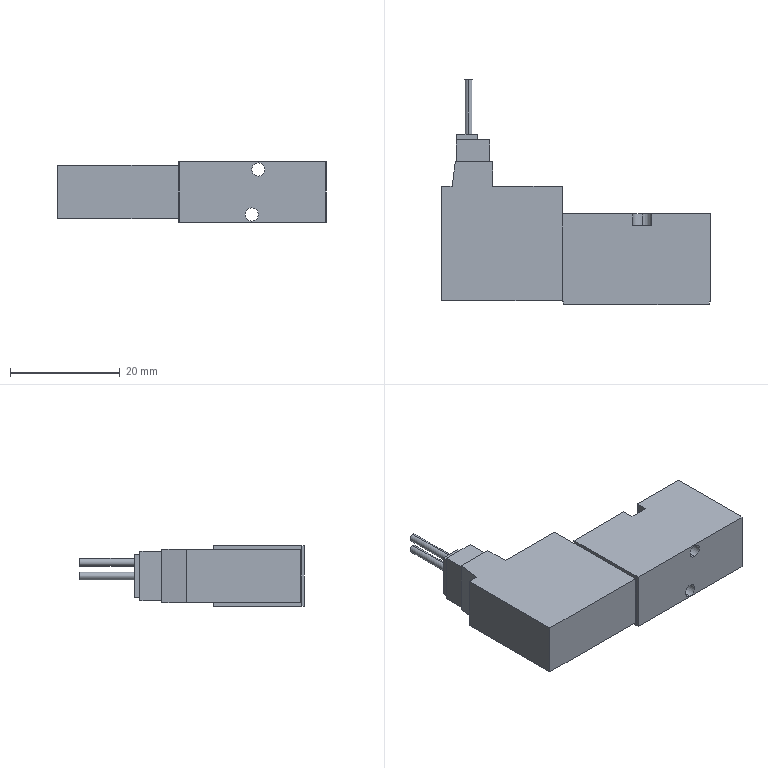Part | SolidWorks | features BaseBody 1, ICE 1 | 1 solid | 49 faces | box 49 x 41 x 11 mm | volume 9805 mm3 | plane 34 | cylinder 11 | spline 4 | commonest cylinder face diameters 1.4 x4 2.4 x4 3.5 x3
STEP:
#1=CARTESIAN_POINT('',(-0.6,14.4,-5.3));
#2=VERTEX_POINT('',#1);
#3=CARTESIAN_POINT('',(-0.6,14.4,-2.9));
#4=VERTEX_POINT('',#3);
#5=CARTESIAN_POINT('',(-0.6,14.4,-4.1));
#6=DIRECTION('',(0.,1.,0.));
#7=DIRECTION('',(0.,0.,-1.));
#8=AXIS2_PLACEMENT_3D('',#5,#6,#7);
#9=CIRCLE('',#8,1.2);
#10=EDGE_CURVE('',#2,#4,#9,.T.);
#11=ORIENTED_EDGE('',*,*,#10,.T.);
#12=CARTESIAN_POINT('',(-0.6,0.,-2.9));
#13=VERTEX_POINT('',#12);
#14=CARTESIAN_POINT('',(-0.6,14.4,-2.9));
#15=DIRECTION('',(0.,-1.,0.));
#16=VECTOR('',#15,1000.);
#17=LINE('',#14,#16);
#18=EDGE_CURVE('',#4,#13,#17,.T.);
#19=ORIENTED_EDGE('',*,*,#18,.T.);
#20=CARTESIAN_POINT('',(-0.6,0.,-5.3));
#21=VERTEX_POINT('',#20);
#22=CARTESIAN_POINT('',(-0.6,0.,-4.1));
#23=DIRECTION('',(0.,1.,0.));
#24=DIRECTION('',(0.,0.,1.));
#25=AXIS2_PLACEMENT_3D('',#22,#23,#24);
#26=CIRCLE('',#25,1.2);
#27=EDGE_CURVE('',#21,#13,#26,.T.);
#28=ORIENTED_EDGE('',*,*,#27,.F.);
#29=CARTESIAN_POINT('',(-0.6,14.4,-5.3));
#30=DIRECTION('',(0.,-1.,0.));
#31=VECTOR('',#30,1000.);
#32=LINE('',#29,#31);
#33=EDGE_CURVE('',#2,#21,#32,.T.);
#34=ORIENTED_EDGE('',*,*,#33,.F.);
#35=EDGE_LOOP('',(#11,#19,#28,#34));
#36=FACE_OUTER_BOUND('',#35,.T.);
#37=CARTESIAN_POINT('',(-0.6,14.4,-4.1));
#38=DIRECTION('',(0.,-1.,0.));
#39=DIRECTION('',(0.,0.,-1.));
#40=AXIS2_PLACEMENT_3D('',#37,#38,#39);
#41=CYLINDRICAL_SURFACE('',#40,1.2);
#42=ADVANCED_FACE('',(#36),#41,.F.);
#43=CARTESIAN_POINT('',(0.6,16.5,2.35));
#44=VERTEX_POINT('',#43);
#45=CARTESIAN_POINT('',(2.35,16.5,4.1));
#46=VERTEX_POINT('',#45);
#47=CARTESIAN_POINT('',(0.6,16.5,4.1));
#48=DIRECTION('',(0.,-1.,0.));
#49=DIRECTION('',(0.,0.,-1.));
#50=AXIS2_PLACEMENT_3D('',#47,#48,#49);
#51=CIRCLE('',#50,1.75);
#52=EDGE_CURVE('',#44,#46,#51,.T.);
#53=ORIENTED_EDGE('',*,*,#52,.F.);
#54=CARTESIAN_POINT('',(0.6,14.4,2.35));
#55=VERTEX_POINT('',#54);
#56=CARTESIAN_POINT('',(0.6,16.5,2.35));
#57=DIRECTION('',(0.,-1.,0.));
#58=VECTOR('',#57,1000.);
#59=LINE('',#56,#58);
#60=EDGE_CURVE('',#44,#55,#59,.T.);
#61=ORIENTED_EDGE('',*,*,#60,.T.);
#62=CARTESIAN_POINT('',(2.35,14.4,4.1));
#63=VERTEX_POINT('',#62);
#64=CARTESIAN_POINT('',(0.6,14.4,4.1));
#65=DIRECTION('',(0.,-1.,0.));
#66=DIRECTION('',(0.,0.,-1.));
#67=AXIS2_PLACEMENT_3D('',#64,#65,#66);
#68=CIRCLE('',#67,1.75);
#69=EDGE_CURVE('',#55,#63,#68,.T.);
#70=ORIENTED_EDGE('',*,*,#69,.T.);
#71=CARTESIAN_POINT('',(2.35,15.45,4.1));
#72=DIRECTION('',(0.,1.,0.));
#73=VECTOR('',#72,1000.);
#74=LINE('',#71,#73);
#75=EDGE_CURVE('',#63,#46,#74,.T.);
#76=ORIENTED_EDGE('',*,*,#75,.T.);
#77=EDGE_LOOP('',(#53,#61,#70,#76));
#78=FACE_OUTER_BOUND('',#77,.T.);
#79=CARTESIAN_POINT('',(0.6,16.5,4.1));
#80=DIRECTION('',(0.,-1.,0.));
#81=DIRECTION('',(0.,0.,-1.));
#82=AXIS2_PLACEMENT_3D('',#79,#80,#81);
#83=CYLINDRICAL_SURFACE('',#82,1.75);
#84=ADVANCED_FACE('',(#78),#83,.F.);
#85=CARTESIAN_POINT('',(0.6,14.4,5.3));
#86=VERTEX_POINT('',#85);
#87=CARTESIAN_POINT('',(0.6,14.4,2.9));
#88=VERTEX_POINT('',#87);
#89=CARTESIAN_POINT('',(0.6,14.4,4.1));
#90=DIRECTION('',(0.,-1.,0.));
#91=DIRECTION('',(0.,0.,-1.));
#92=AXIS2_PLACEMENT_3D('',#89,#90,#91);
#93=CIRCLE('',#92,1.2);
#94=EDGE_CURVE('',#86,#88,#93,.T.);
#95=ORIENTED_EDGE('',*,*,#94,.F.);
#96=CARTESIAN_POINT('',(0.6,0.,5.3));
#97=VERTEX_POINT('',#96);
#98=CARTESIAN_POINT('',(0.6,14.4,5.3));
#99=DIRECTION('',(0.,-1.,0.));
#100=VECTOR('',#99,1000.);
#101=LINE('',#98,#100);
#102=EDGE_CURVE('',#86,#97,#101,.T.);
#103=ORIENTED_EDGE('',*,*,#102,.T.);
#104=CARTESIAN_POINT('',(0.6,0.,2.9));
#105=VERTEX_POINT('',#104);
#106=CARTESIAN_POINT('',(0.6,0.,4.1));
#107=DIRECTION('',(0.,1.,0.));
#108=DIRECTION('',(0.,0.,1.));
#109=AXIS2_PLACEMENT_3D('',#106,#107,#108);
#110=CIRCLE('',#109,1.2);
#111=EDGE_CURVE('',#105,#97,#110,.T.);
#112=ORIENTED_EDGE('',*,*,#111,.F.);
#113=CARTESIAN_POINT('',(0.6,14.4,2.9));
#114=DIRECTION('',(0.,-1.,0.));
#115=VECTOR('',#114,1000.);
#116=LINE('',#113,#115);
#117=EDGE_CURVE('',#88,#105,#116,.T.);
#118=ORIENTED_EDGE('',*,*,#117,.F.);
#119=EDGE_LOOP('',(#95,#103,#112,#118));
#120=FACE_OUTER_BOUND('',#119,.T.);
#121=CARTESIAN_POINT('',(0.6,14.4,4.1));
#122=DIRECTION('',(0.,-1.,0.));
#123=DIRECTION('',(0.,0.,-1.));
#124=AXIS2_PLACEMENT_3D('',#121,#122,#123);
#125=CYLINDRICAL_SURFACE('',#124,1.2);
#126=ADVANCED_FACE('',(#120),#125,.F.);
#127=CARTESIAN_POINT('',(-31.07,31.,-0.7));
#128=VERTEX_POINT('',#127);
#129=CARTESIAN_POINT('',(-31.07,31.,0.7));
#130=VERTEX_POINT('',#129);
#131=CARTESIAN_POINT('',(-31.07,31.,0.));
#132=DIRECTION('',(0.,-1.,0.));
#133=DIRECTION('',(0.,0.,1.));
#134=AXIS2_PLACEMENT_3D('',#131,#132,#133);
#135=CIRCLE('',#134,0.7);
#136=EDGE_CURVE('',#128,#130,#135,.T.);
#137=ORIENTED_EDGE('',*,*,#136,.F.);
#138=CARTESIAN_POINT('',(-31.07,41.,-0.7));
#139=VERTEX_POINT('',#138);
#140=CARTESIAN_POINT('',(-31.07,41.,-0.7));
#141=DIRECTION('',(0.,1.,0.));
#142=VECTOR('',#141,1000.);
#143=LINE('',#140,#142);
#144=EDGE_CURVE('',#128,#139,#143,.T.);
#145=ORIENTED_EDGE('',*,*,#144,.T.);
#146=CARTESIAN_POINT('',(-31.07,41.,0.7));
#147=VERTEX_POINT('',#146);
#148=CARTESIAN_POINT('',(-31.07,41.,0.));
#149=DIRECTION('',(0.,-1.,0.));
#150=DIRECTION('',(0.,0.,1.));
#151=AXIS2_PLACEMENT_3D('',#148,#149,#150);
#152=CIRCLE('',#151,0.7);
#153=EDGE_CURVE('',#139,#147,#152,.T.);
#154=ORIENTED_EDGE('',*,*,#153,.T.);
#155=CARTESIAN_POINT('',(-31.07,41.,0.7));
#156=DIRECTION('',(0.,1.,0.));
#157=VECTOR('',#156,1000.);
#158=LINE('',#155,#157);
#159=EDGE_CURVE('',#130,#147,#158,.T.);
#160=ORIENTED_EDGE('',*,*,#159,.F.);
#161=EDGE_LOOP('',(#137,#145,#154,#160));
#162=FACE_OUTER_BOUND('',#161,.T.);
#163=CARTESIAN_POINT('',(-31.07,41.,0.));
#164=DIRECTION('',(0.,1.,0.));
#165=DIRECTION('',(0.,0.,1.));
#166=AXIS2_PLACEMENT_3D('',#163,#164,#165);
#167=CYLINDRICAL_SURFACE('',#166,0.7);
#168=ADVANCED_FACE('',(#162),#167,.T.);
#169=CARTESIAN_POINT('',(-31.07,31.,1.8));
#170=VERTEX_POINT('',#169);
#171=CARTESIAN_POINT('',(-31.07,31.,3.2));
#172=VERTEX_POINT('',#171);
#173=CARTESIAN_POINT('',(-31.07,31.,2.5));
#174=DIRECTION('',(0.,-1.,0.));
#175=DIRECTION('',(0.,0.,1.));
#176=AXIS2_PLACEMENT_3D('',#173,#174,#175);
#177=CIRCLE('',#176,0.7);
#178=EDGE_CURVE('',#170,#172,#177,.T.);
#179=ORIENTED_EDGE('',*,*,#178,.F.);
#180=CARTESIAN_POINT('',(-31.07,41.,1.8));
#181=VERTEX_POINT('',#180);
#182=CARTESIAN_POINT('',(-31.07,41.,1.8));
#183=DIRECTION('',(0.,1.,0.));
#184=VECTOR('',#183,1000.);
#185=LINE('',#182,#184);
#186=EDGE_CURVE('',#170,#181,#185,.T.);
#187=ORIENTED_EDGE('',*,*,#186,.T.);
#188=CARTESIAN_POINT('',(-31.07,41.,3.2));
#189=VERTEX_POINT('',#188);
#190=CARTESIAN_POINT('',(-31.07,41.,2.5));
#191=DIRECTION('',(0.,-1.,0.));
#192=DIRECTION('',(0.,0.,1.));
#193=AXIS2_PLACEMENT_3D('',#190,#191,#192);
#194=CIRCLE('',#193,0.7);
#195=EDGE_CURVE('',#181,#189,#194,.T.);
#196=ORIENTED_EDGE('',*,*,#195,.T.);
#197=CARTESIAN_POINT('',(-31.07,41.,3.2));
#198=DIRECTION('',(0.,1.,0.));
#199=VECTOR('',#198,1000.);
#200=LINE('',#197,#199);
#201=EDGE_CURVE('',#172,#189,#200,.T.);
#202=ORIENTED_EDGE('',*,*,#201,.F.);
#203=EDGE_LOOP('',(#179,#187,#196,#202));
#204=FACE_OUTER_BOUND('',#203,.T.);
#205=CARTESIAN_POINT('',(-31.07,41.,2.5));
#206=DIRECTION('',(0.,1.,0.));
#207=DIRECTION('',(0.,0.,1.));
#208=AXIS2_PLACEMENT_3D('',#205,#206,#207);
#209=CYLINDRICAL_SURFACE('',#208,0.7);
#210=ADVANCED_FACE('',(#204),#209,.T.);
#211=ORIENTED_EDGE('',*,*,#18,.F.);
#212=CARTESIAN_POINT('',(-0.6,14.4,-4.1));
#213=DIRECTION('',(0.,1.,0.));
#214=DIRECTION('',(0.,0.,-1.));
#215=AXIS2_PLACEMENT_3D('',#212,#213,#214);
#216=CIRCLE('',#215,1.2);
#217=EDGE_CURVE('',#4,#2,#216,.T.);
#218=ORIENTED_EDGE('',*,*,#217,.T.);
#219=ORIENTED_EDGE('',*,*,#33,.T.);
#220=CARTESIAN_POINT('',(-0.6,0.,-4.1));
#221=DIRECTION('',(0.,1.,0.));
#222=DIRECTION('',(0.,0.,1.));
#223=AXIS2_PLACEMENT_3D('',#220,#221,#222);
#224=CIRCLE('',#223,1.2);
#225=EDGE_CURVE('',#13,#21,#224,.T.);
#226=ORIENTED_EDGE('',*,*,#225,.F.);
#227=EDGE_LOOP('',(#211,#218,#219,#226));
#228=FACE_OUTER_BOUND('',#227,.T.);
#229=CARTESIAN_POINT('',(-0.6,14.4,-4.1));
#230=DIRECTION('',(0.,-1.,0.));
#231=DIRECTION('',(0.,0.,-1.));
#232=AXIS2_PLACEMENT_3D('',#229,#230,#231);
#233=CYLINDRICAL_SURFACE('',#232,1.2);
#234=ADVANCED_FACE('',(#228),#233,.F.);
#235=ORIENTED_EDGE('',*,*,#10,.F.);
#236=ORIENTED_EDGE('',*,*,#217,.F.);
#237=EDGE_LOOP('',(#235,#236));
#238=FACE_BOUND('',#237,.T.);
#239=CARTESIAN_POINT('',(1.15,14.4,-5.5));
#240=VERTEX_POINT('',#239);
#241=CARTESIAN_POINT('',(-2.35,14.4,-5.5));
#242=VERTEX_POINT('',#241);
#243=CARTESIAN_POINT('',(-2.35,14.4,-5.5));
#244=DIRECTION('',(-1.,0.,0.));
#245=VECTOR('',#244,1000.);
#246=LINE('',#243,#245);
#247=EDGE_CURVE('',#240,#242,#246,.T.);
#248=ORIENTED_EDGE('',*,*,#247,.T.);
#249=CARTESIAN_POINT('',(-2.35,14.4,-4.1));
#250=VERTEX_POINT('',#249);
#251=CARTESIAN_POINT('',(-2.35,14.4,-4.8));
#252=DIRECTION('',(0.,0.,-1.));
#253=VECTOR('',#252,1000.);
#254=LINE('',#251,#253);
#255=EDGE_CURVE('',#250,#242,#254,.T.);
#256=ORIENTED_EDGE('',*,*,#255,.F.);
#257=CARTESIAN_POINT('',(1.15,14.4,-4.1));
#258=VERTEX_POINT('',#257);
#259=CARTESIAN_POINT('',(-0.6,14.4,-4.1));
#260=DIRECTION('',(0.,1.,0.));
#261=DIRECTION('',(0.,0.,-1.));
#262=AXIS2_PLACEMENT_3D('',#259,#260,#261);
#263=CIRCLE('',#262,1.75);
#264=EDGE_CURVE('',#250,#258,#263,.T.);
#265=ORIENTED_EDGE('',*,*,#264,.T.);
#266=CARTESIAN_POINT('',(1.15,14.4,-4.8));
#267=DIRECTION('',(0.,0.,1.));
#268=VECTOR('',#267,1000.);
#269=LINE('',#266,#268);
#270=EDGE_CURVE('',#240,#258,#269,.T.);
#271=ORIENTED_EDGE('',*,*,#270,.F.);
#272=EDGE_LOOP('',(#248,#256,#265,#271));
#273=FACE_OUTER_BOUND('',#272,.T.);
#274=CARTESIAN_POINT('',(-2.35,14.4,-5.5));
#275=CARTESIAN_POINT('',(1.15,14.4,-5.5));
#276=CARTESIAN_POINT('',(-2.35,14.4,-2.35));
#277=CARTESIAN_POINT('',(1.15,14.4,-2.35));
#278=CARTESIAN_POINT('',(-2.35,14.4,-2.322));
#279=CARTESIAN_POINT('',(1.15,14.4,-2.322));
#280=B_SPLINE_SURFACE_WITH_KNOTS('',1,1,((#274,#275),(#276,#277),(#278,#279)),.UNSPECIFIED.,.F.,.F.,.F.,(2,1,2),(2,2),(0.,1.,1.009),(0.,1.),.UNSPECIFIED.);
#281=ADVANCED_FACE('',(#238,#273),#280,.T.);
#282=CARTESIAN_POINT('',(-14.,0.5,-5.5));
#283=VERTEX_POINT('',#282);
#284=CARTESIAN_POINT('',(-14.,16.5,-5.5));
#285=VERTEX_POINT('',#284);
#286=CARTESIAN_POINT('',(-14.,0.,-5.5));
#287=DIRECTION('',(0.,1.,0.));
#288=VECTOR('',#287,1000.);
#289=LINE('',#286,#288);
#290=EDGE_CURVE('',#283,#285,#289,.T.);
#291=ORIENTED_EDGE('',*,*,#290,.T.);
#292=CARTESIAN_POINT('',(-2.35,16.5,-5.5));
#293=VERTEX_POINT('',#292);
#294=CARTESIAN_POINT('',(-0.5,16.5,-5.5));
#295=DIRECTION('',(1.,0.,0.));
#296=VECTOR('',#295,1000.);
#297=LINE('',#294,#296);
#298=EDGE_CURVE('',#285,#293,#297,.T.);
#299=ORIENTED_EDGE('',*,*,#298,.T.);
#300=CARTESIAN_POINT('',(-2.35,0.,-5.5));
#301=DIRECTION('',(0.,-1.,0.));
#302=VECTOR('',#301,1000.);
#303=LINE('',#300,#302);
#304=EDGE_CURVE('',#293,#242,#303,.T.);
#305=ORIENTED_EDGE('',*,*,#304,.T.);
#306=ORIENTED_EDGE('',*,*,#247,.F.);
#307=CARTESIAN_POINT('',(1.15,16.5,-5.5));
#308=VERTEX_POINT('',#307);
#309=CARTESIAN_POINT('',(1.15,0.,-5.5));
#310=DIRECTION('',(0.,1.,0.));
#311=VECTOR('',#310,1000.);
#312=LINE('',#309,#311);
#313=EDGE_CURVE('',#240,#308,#312,.T.);
#314=ORIENTED_EDGE('',*,*,#313,.T.);
#315=CARTESIAN_POINT('',(13.,16.5,-5.5));
#316=VERTEX_POINT('',#315);
#317=CARTESIAN_POINT('',(-0.5,16.5,-5.5));
#318=DIRECTION('',(1.,0.,0.));
#319=VECTOR('',#318,1000.);
#320=LINE('',#317,#319);
#321=EDGE_CURVE('',#308,#316,#320,.T.);
#322=ORIENTED_EDGE('',*,*,#321,.T.);
#323=CARTESIAN_POINT('',(13.,0.5,-5.5));
#324=VERTEX_POINT('',#323);
#325=CARTESIAN_POINT('',(13.,0.,-5.5));
#326=DIRECTION('',(0.,-1.,0.));
#327=VECTOR('',#326,1000.);
#328=LINE('',#325,#327);
#329=EDGE_CURVE('',#316,#324,#328,.T.);
#330=ORIENTED_EDGE('',*,*,#329,.T.);
#331=CARTESIAN_POINT('',(12.8,0.5,-5.5));
#332=VERTEX_POINT('',#331);
#333=CARTESIAN_POINT('',(12.9,0.5,-5.5));
#334=DIRECTION('',(1.,0.,0.));
#335=VECTOR('',#334,1000.);
#336=LINE('',#333,#335);
#337=EDGE_CURVE('',#332,#324,#336,.T.);
#338=ORIENTED_EDGE('',*,*,#337,.F.);
#339=CARTESIAN_POINT('',(12.8,0.,-5.5));
#340=VERTEX_POINT('',#339);
#341=CARTESIAN_POINT('',(12.8,0.25,-5.5));
#342=DIRECTION('',(0.,1.,0.));
#343=VECTOR('',#342,1000.);
#344=LINE('',#341,#343);
#345=EDGE_CURVE('',#340,#332,#344,.T.);
#346=ORIENTED_EDGE('',*,*,#345,.F.);
#347=CARTESIAN_POINT('',(-13.8,0.,-5.5));
#348=VERTEX_POINT('',#347);
#349=CARTESIAN_POINT('',(-0.5,0.,-5.5));
#350=DIRECTION('',(-1.,0.,0.));
#351=VECTOR('',#350,1000.);
#352=LINE('',#349,#351);
#353=EDGE_CURVE('',#340,#348,#352,.T.);
#354=ORIENTED_EDGE('',*,*,#353,.T.);
#355=CARTESIAN_POINT('',(-13.8,0.5,-5.5));
#356=VERTEX_POINT('',#355);
#357=CARTESIAN_POINT('',(-13.8,0.25,-5.5));
#358=DIRECTION('',(0.,-1.,0.));
#359=VECTOR('',#358,1000.);
#360=LINE('',#357,#359);
#361=EDGE_CURVE('',#356,#348,#360,.T.);
#362=ORIENTED_EDGE('',*,*,#361,.F.);
#363=CARTESIAN_POINT('',(-13.9,0.5,-5.5));
#364=DIRECTION('',(1.,0.,0.));
#365=VECTOR('',#364,1000.);
#366=LINE('',#363,#365);
#367=EDGE_CURVE('',#283,#356,#366,.T.);
#368=ORIENTED_EDGE('',*,*,#367,.F.);
#369=EDGE_LOOP('',(#291,#299,#305,#306,#314,#322,#330,#338,#346,#354,#362,#368));
#370=FACE_OUTER_BOUND('',#369,.T.);
#371=CARTESIAN_POINT('',(13.,0.,-5.5));
#372=DIRECTION('',(0.,0.,-1.));
#373=DIRECTION('',(-1.,0.,0.));
#374=AXIS2_PLACEMENT_3D('',#371,#372,#373);
#375=PLANE('',#374);
#376=ADVANCED_FACE('',(#370),#375,.T.);
#377=CARTESIAN_POINT('',(-2.35,16.5,-4.1));
#378=VERTEX_POINT('',#377);
#379=CARTESIAN_POINT('',(1.15,16.5,-4.1));
#380=VERTEX_POINT('',#379);
#381=CARTESIAN_POINT('',(-0.6,16.5,-4.1));
#382=DIRECTION('',(0.,1.,0.));
#383=DIRECTION('',(0.,0.,-1.));
#384=AXIS2_PLACEMENT_3D('',#381,#382,#383);
#385=CIRCLE('',#384,1.75);
#386=EDGE_CURVE('',#378,#380,#385,.T.);
#387=ORIENTED_EDGE('',*,*,#386,.T.);
#388=CARTESIAN_POINT('',(1.15,15.45,-4.1));
#389=DIRECTION('',(0.,-1.,0.));
#390=VECTOR('',#389,1000.);
#391=LINE('',#388,#390);
#392=EDGE_CURVE('',#380,#258,#391,.T.);
#393=ORIENTED_EDGE('',*,*,#392,.T.);
#394=ORIENTED_EDGE('',*,*,#264,.F.);
#395=CARTESIAN_POINT('',(-2.35,15.45,-4.1));
#396=DIRECTION('',(0.,1.,0.));
#397=VECTOR('',#396,1000.);
#398=LINE('',#395,#397);
#399=EDGE_CURVE('',#250,#378,#398,.T.);
#400=ORIENTED_EDGE('',*,*,#399,.T.);
#401=EDGE_LOOP('',(#387,#393,#394,#400));
#402=FACE_OUTER_BOUND('',#401,.T.);
#403=CARTESIAN_POINT('',(-0.6,16.5,-4.1));
#404=DIRECTION('',(0.,-1.,0.));
#405=DIRECTION('',(0.,0.,-1.));
#406=AXIS2_PLACEMENT_3D('',#403,#404,#405);
#407=CYLINDRICAL_SURFACE('',#406,1.75);
#408=ADVANCED_FACE('',(#402),#407,.F.);
#409=CARTESIAN_POINT('',(-14.,16.5,4.9));
#410=VERTEX_POINT('',#409);
#411=CARTESIAN_POINT('',(-14.,16.5,5.5));
#412=VERTEX_POINT('',#411);
#413=CARTESIAN_POINT('',(-14.,16.5,5.5));
#414=DIRECTION('',(0.,0.,1.));
#415=VECTOR('',#414,1000.);
#416=LINE('',#413,#415);
#417=EDGE_CURVE('',#410,#412,#416,.T.);
#418=ORIENTED_EDGE('',*,*,#417,.T.);
#419=CARTESIAN_POINT('',(-1.15,16.5,5.5));
#420=VERTEX_POINT('',#419);
#421=CARTESIAN_POINT('',(-0.5,16.5,5.5));
#422=DIRECTION('',(1.,0.,0.));
#423=VECTOR('',#422,1000.);
#424=LINE('',#421,#423);
#425=EDGE_CURVE('',#412,#420,#424,.T.);
#426=ORIENTED_EDGE('',*,*,#425,.T.);
#427=CARTESIAN_POINT('',(-1.15,16.5,4.1));
#428=VERTEX_POINT('',#427);
#429=CARTESIAN_POINT('',(-1.15,16.5,4.8));
#430=DIRECTION('',(0.,0.,1.));
#431=VECTOR('',#430,1000.);
#432=LINE('',#429,#431);
#433=EDGE_CURVE('',#428,#420,#432,.T.);
#434=ORIENTED_EDGE('',*,*,#433,.F.);
#435=CARTESIAN_POINT('',(0.6,16.5,4.1));
#436=DIRECTION('',(0.,-1.,0.));
#437=DIRECTION('',(0.,0.,-1.));
#438=AXIS2_PLACEMENT_3D('',#435,#436,#437);
#439=CIRCLE('',#438,1.75);
#440=EDGE_CURVE('',#428,#44,#439,.T.);
#441=ORIENTED_EDGE('',*,*,#440,.T.);
#442=ORIENTED_EDGE('',*,*,#52,.T.);
#443=CARTESIAN_POINT('',(2.35,16.5,5.5));
#444=VERTEX_POINT('',#443);
#445=CARTESIAN_POINT('',(2.35,16.5,4.8));
#446=DIRECTION('',(0.,0.,-1.));
#447=VECTOR('',#446,1000.);
#448=LINE('',#445,#447);
#449=EDGE_CURVE('',#444,#46,#448,.T.);
#450=ORIENTED_EDGE('',*,*,#449,.F.);
#451=CARTESIAN_POINT('',(13.,16.5,5.5));
#452=VERTEX_POINT('',#451);
#453=CARTESIAN_POINT('',(-0.5,16.5,5.5));
#454=DIRECTION('',(1.,0.,0.));
#455=VECTOR('',#454,1000.);
#456=LINE('',#453,#455);
#457=EDGE_CURVE('',#444,#452,#456,.T.);
#458=ORIENTED_EDGE('',*,*,#457,.T.);
#459=CARTESIAN_POINT('',(13.,16.5,5.5));
#460=DIRECTION('',(0.,0.,-1.));
#461=VECTOR('',#460,1000.);
#462=LINE('',#459,#461);
#463=EDGE_CURVE('',#452,#316,#462,.T.);
#464=ORIENTED_EDGE('',*,*,#463,.T.);
#465=ORIENTED_EDGE('',*,*,#321,.F.);
#466=CARTESIAN_POINT('',(1.15,16.5,5.5));
#467=DIRECTION('',(0.,0.,1.));
#468=VECTOR('',#467,1000.);
#469=LINE('',#466,#468);
#470=EDGE_CURVE('',#308,#380,#469,.T.);
#471=ORIENTED_EDGE('',*,*,#470,.T.);
#472=ORIENTED_EDGE('',*,*,#386,.F.);
#473=CARTESIAN_POINT('',(-2.35,16.5,5.5));
#474=DIRECTION('',(0.,0.,-1.));
#475=VECTOR('',#474,1000.);
#476=LINE('',#473,#475);
#477=EDGE_CURVE('',#378,#293,#476,.T.);
#478=ORIENTED_EDGE('',*,*,#477,.T.);
#479=ORIENTED_EDGE('',*,*,#298,.F.);
#480=CARTESIAN_POINT('',(-14.,16.5,-4.9));
#481=VERTEX_POINT('',#480);
#482=CARTESIAN_POINT('',(-14.,16.5,5.5));
#483=DIRECTION('',(0.,0.,1.));
#484=VECTOR('',#483,1000.);
#485=LINE('',#482,#484);
#486=EDGE_CURVE('',#285,#481,#485,.T.);
#487=ORIENTED_EDGE('',*,*,#486,.T.);
#488=CARTESIAN_POINT('',(-14.,16.5,5.5));
#489=DIRECTION('',(0.,0.,1.));
#490=VECTOR('',#489,1000.);
#491=LINE('',#488,#490);
#492=EDGE_CURVE('',#481,#410,#491,.T.);
#493=ORIENTED_EDGE('',*,*,#492,.T.);
#494=EDGE_LOOP('',(#418,#426,#434,#441,#442,#450,#458,#464,#465,#471,#472,#478,#479,#487,#493));
#495=FACE_OUTER_BOUND('',#494,.T.);
#496=CARTESIAN_POINT('',(-14.,16.5,5.5));
#497=DIRECTION('',(0.,1.,0.));
#498=DIRECTION('',(1.,0.,0.));
#499=AXIS2_PLACEMENT_3D('',#496,#497,#498);
#500=PLANE('',#499);
#501=ADVANCED_FACE('',(#495),#500,.T.);
#502=CARTESIAN_POINT('',(-14.,0.5,5.5));
#503=VERTEX_POINT('',#502);
#504=CARTESIAN_POINT('',(-14.,8.5,5.5));
#505=DIRECTION('',(0.,1.,0.));
#506=VECTOR('',#505,1000.);
#507=LINE('',#504,#506);
#508=EDGE_CURVE('',#503,#412,#507,.T.);
#509=ORIENTED_EDGE('',*,*,#508,.T.);
#510=ORIENTED_EDGE('',*,*,#417,.F.);
#511=CARTESIAN_POINT('',(-14.,0.7,4.9));
#512=VERTEX_POINT('',#511);
#513=CARTESIAN_POINT('',(-14.,8.5,4.9));
#514=DIRECTION('',(0.,-1.,0.));
#515=VECTOR('',#514,1000.);
#516=LINE('',#513,#515);
#517=EDGE_CURVE('',#410,#512,#516,.T.);
#518=ORIENTED_EDGE('',*,*,#517,.T.);
#519=CARTESIAN_POINT('',(-14.,0.7,-4.9));
#520=VERTEX_POINT('',#519);
#521=CARTESIAN_POINT('',(-14.,0.7,5.5));
#522=DIRECTION('',(0.,0.,-1.));
#523=VECTOR('',#522,1000.);
#524=LINE('',#521,#523);
#525=EDGE_CURVE('',#512,#520,#524,.T.);
#526=ORIENTED_EDGE('',*,*,#525,.T.);
#527=CARTESIAN_POINT('',(-14.,8.5,-4.9));
#528=DIRECTION('',(0.,1.,0.));
#529=VECTOR('',#528,1000.);
#530=LINE('',#527,#529);
#531=EDGE_CURVE('',#520,#481,#530,.T.);
#532=ORIENTED_EDGE('',*,*,#531,.T.);
#533=ORIENTED_EDGE('',*,*,#486,.F.);
#534=ORIENTED_EDGE('',*,*,#290,.F.);
#535=CARTESIAN_POINT('',(-14.,0.5,5.5));
#536=DIRECTION('',(0.,0.,1.));
#537=VECTOR('',#536,1000.);
#538=LINE('',#535,#537);
#539=EDGE_CURVE('',#283,#503,#538,.T.);
#540=ORIENTED_EDGE('',*,*,#539,.T.);
#541=EDGE_LOOP('',(#509,#510,#518,#526,#532,#533,#534,#540));
#542=FACE_OUTER_BOUND('',#541,.T.);
#543=CARTESIAN_POINT('',(-14.,0.5,5.5));
#544=DIRECTION('',(-1.,0.,0.));
#545=DIRECTION('',(0.,1.,0.));
#546=AXIS2_PLACEMENT_3D('',#543,#544,#545);
#547=PLANE('',#546);
#548=ADVANCED_FACE('',(#542),#547,.T.);
#549=ORIENTED_EDGE('',*,*,#353,.F.);
#550=CARTESIAN_POINT('',(12.8,0.,5.5));
#551=VERTEX_POINT('',#550);
#552=CARTESIAN_POINT('',(12.8,0.,5.5));
#553=DIRECTION('',(0.,0.,1.));
#554=VECTOR('',#553,1000.);
#555=LINE('',#552,#554);
#556=EDGE_CURVE('',#340,#551,#555,.T.);
#557=ORIENTED_EDGE('',*,*,#556,.T.);
#558=CARTESIAN_POINT('',(-13.8,0.,5.5));
#559=VERTEX_POINT('',#558);
#560=CARTESIAN_POINT('',(-0.5,0.,5.5));
#561=DIRECTION('',(1.,0.,0.));
#562=VECTOR('',#561,1000.);
#563=LINE('',#560,#562);
#564=EDGE_CURVE('',#559,#551,#563,.T.);
#565=ORIENTED_EDGE('',*,*,#564,.F.);
#566=CARTESIAN_POINT('',(-13.8,0.,5.5));
#567=DIRECTION('',(0.,0.,-1.));
#568=VECTOR('',#567,1000.);
#569=LINE('',#566,#568);
#570=EDGE_CURVE('',#559,#348,#569,.T.);
#571=ORIENTED_EDGE('',*,*,#570,.T.);
#572=EDGE_LOOP('',(#549,#557,#565,#571));
#573=FACE_OUTER_BOUND('',#572,.T.);
#574=ORIENTED_EDGE('',*,*,#111,.T.);
#575=CARTESIAN_POINT('',(0.6,0.,4.1));
#576=DIRECTION('',(0.,1.,0.));
#577=DIRECTION('',(0.,0.,1.));
#578=AXIS2_PLACEMENT_3D('',#575,#576,#577);
#579=CIRCLE('',#578,1.2);
#580=EDGE_CURVE('',#97,#105,#579,.T.);
#581=ORIENTED_EDGE('',*,*,#580,.T.);
#582=EDGE_LOOP('',(#574,#581));
#583=FACE_BOUND('',#582,.T.);
#584=ORIENTED_EDGE('',*,*,#27,.T.);
#585=ORIENTED_EDGE('',*,*,#225,.T.);
#586=EDGE_LOOP('',(#584,#585));
#587=FACE_BOUND('',#586,.T.);
#588=CARTESIAN_POINT('',(12.8,0.,-5.4));
#589=DIRECTION('',(0.,-1.,0.));
#590=DIRECTION('',(-1.,0.,0.));
#591=AXIS2_PLACEMENT_3D('',#588,#589,#590);
#592=PLANE('',#591);
#593=ADVANCED_FACE('',(#573,#583,#587),#592,.T.);
#594=CARTESIAN_POINT('',(13.,0.5,5.5));
#595=VERTEX_POINT('',#594);
#596=CARTESIAN_POINT('',(13.,8.5,5.5));
#597=DIRECTION('',(0.,-1.,0.));
#598=VECTOR('',#597,1000.);
#599=LINE('',#596,#598);
#600=EDGE_CURVE('',#452,#595,#599,.T.);
#601=ORIENTED_EDGE('',*,*,#600,.T.);
#602=CARTESIAN_POINT('',(13.,0.5,5.5));
#603=DIRECTION('',(0.,0.,-1.));
#604=VECTOR('',#603,1000.);
#605=LINE('',#602,#604);
#606=EDGE_CURVE('',#595,#324,#605,.T.);
#607=ORIENTED_EDGE('',*,*,#606,.T.);
#608=ORIENTED_EDGE('',*,*,#329,.F.);
#609=ORIENTED_EDGE('',*,*,#463,.F.);
#610=EDGE_LOOP('',(#601,#607,#608,#609));
#611=FACE_OUTER_BOUND('',#610,.T.);
#612=CARTESIAN_POINT('',(13.,16.5,5.5));
#613=DIRECTION('',(1.,0.,0.));
#614=DIRECTION('',(0.,-1.,0.));
#615=AXIS2_PLACEMENT_3D('',#612,#613,#614);
#616=PLANE('',#615);
#617=ADVANCED_FACE('',(#611),#616,.T.);
#618=ORIENTED_EDGE('',*,*,#470,.F.);
#619=ORIENTED_EDGE('',*,*,#313,.F.);
#620=ORIENTED_EDGE('',*,*,#270,.T.);
#621=ORIENTED_EDGE('',*,*,#392,.F.);
#622=EDGE_LOOP('',(#618,#619,#620,#621));
#623=FACE_OUTER_BOUND('',#622,.T.);
#624=CARTESIAN_POINT('',(1.15,16.5,-4.1));
#625=DIRECTION('',(-1.,0.,0.));
#626=DIRECTION('',(0.,0.,-1.));
#627=AXIS2_PLACEMENT_3D('',#624,#625,#626);
#628=PLANE('',#627);
#629=ADVANCED_FACE('',(#623),#628,.T.);
#630=ORIENTED_EDGE('',*,*,#477,.F.);
#631=ORIENTED_EDGE('',*,*,#399,.F.);
#632=ORIENTED_EDGE('',*,*,#255,.T.);
#633=ORIENTED_EDGE('',*,*,#304,.F.);
#634=EDGE_LOOP('',(#630,#631,#632,#633));
#635=FACE_OUTER_BOUND('',#634,.T.);
#636=CARTESIAN_POINT('',(-2.35,16.5,-5.5));
#637=DIRECTION('',(1.,0.,0.));
#638=DIRECTION('',(0.,0.,1.));
#639=AXIS2_PLACEMENT_3D('',#636,#637,#638);
#640=PLANE('',#639);
#641=ADVANCED_FACE('',(#635),#640,.T.);
#642=CARTESIAN_POINT('',(2.35,14.4,5.5));
#643=VERTEX_POINT('',#642);
#644=CARTESIAN_POINT('',(2.35,0.,5.5));
#645=DIRECTION('',(0.,-1.,0.));
#646=VECTOR('',#645,1000.);
#647=LINE('',#644,#646);
#648=EDGE_CURVE('',#444,#643,#647,.T.);
#649=ORIENTED_EDGE('',*,*,#648,.T.);
#650=CARTESIAN_POINT('',(-1.15,14.4,5.5));
#651=VERTEX_POINT('',#650);
#652=CARTESIAN_POINT('',(-0.5,14.4,5.5));
#653=DIRECTION('',(-1.,0.,0.));
#654=VECTOR('',#653,1000.);
#655=LINE('',#652,#654);
#656=EDGE_CURVE('',#643,#651,#655,.T.);
#657=ORIENTED_EDGE('',*,*,#656,.T.);
#658=CARTESIAN_POINT('',(-1.15,0.,5.5));
#659=DIRECTION('',(0.,1.,0.));
#660=VECTOR('',#659,1000.);
#661=LINE('',#658,#660);
#662=EDGE_CURVE('',#651,#420,#661,.T.);
#663=ORIENTED_EDGE('',*,*,#662,.T.);
#664=ORIENTED_EDGE('',*,*,#425,.F.);
#665=ORIENTED_EDGE('',*,*,#508,.F.);
#666=CARTESIAN_POINT('',(-13.8,0.5,5.5));
#667=VERTEX_POINT('',#666);
#668=CARTESIAN_POINT('',(-0.5,0.5,5.5));
#669=DIRECTION('',(1.,0.,0.));
#670=VECTOR('',#669,1000.);
#671=LINE('',#668,#670);
#672=EDGE_CURVE('',#503,#667,#671,.T.);
#673=ORIENTED_EDGE('',*,*,#672,.T.);
#674=CARTESIAN_POINT('',(-13.8,0.25,5.5));
#675=DIRECTION('',(0.,1.,0.));
#676=VECTOR('',#675,1000.);
#677=LINE('',#674,#676);
#678=EDGE_CURVE('',#559,#667,#677,.T.);
#679=ORIENTED_EDGE('',*,*,#678,.F.);
#680=ORIENTED_EDGE('',*,*,#564,.T.);
#681=CARTESIAN_POINT('',(12.8,0.5,5.5));
#682=VERTEX_POINT('',#681);
#683=CARTESIAN_POINT('',(12.8,0.25,5.5));
#684=DIRECTION('',(0.,-1.,0.));
#685=VECTOR('',#684,1000.);
#686=LINE('',#683,#685);
#687=EDGE_CURVE('',#682,#551,#686,.T.);
#688=ORIENTED_EDGE('',*,*,#687,.F.);
#689=CARTESIAN_POINT('',(-0.5,0.5,5.5));
#690=DIRECTION('',(1.,0.,0.));
#691=VECTOR('',#690,1000.);
#692=LINE('',#689,#691);
#693=EDGE_CURVE('',#682,#595,#692,.T.);
#694=ORIENTED_EDGE('',*,*,#693,.T.);
#695=ORIENTED_EDGE('',*,*,#600,.F.);
#696=ORIENTED_EDGE('',*,*,#457,.F.);
#697=EDGE_LOOP('',(#649,#657,#663,#664,#665,#673,#679,#680,#688,#694,#695,#696));
#698=FACE_OUTER_BOUND('',#697,.T.);
#699=CARTESIAN_POINT('',(-14.,0.,5.5));
#700=DIRECTION('',(0.,0.,1.));
#701=DIRECTION('',(1.,0.,0.));
#702=AXIS2_PLACEMENT_3D('',#699,#700,#701);
#703=PLANE('',#702);
#704=ADVANCED_FACE('',(#698),#703,.T.);
#705=CARTESIAN_POINT('',(-14.,21.5,-4.9));
#706=VERTEX_POINT('',#705);
#707=CARTESIAN_POINT('',(-14.,21.5,4.9));
#708=VERTEX_POINT('',#707);
#709=CARTESIAN_POINT('',(-14.,21.5,4.9));
#710=DIRECTION('',(0.,0.,1.));
#711=VECTOR('',#710,1000.);
#712=LINE('',#709,#711);
#713=EDGE_CURVE('',#706,#708,#712,.T.);
#714=ORIENTED_EDGE('',*,*,#713,.T.);
#715=CARTESIAN_POINT('',(-14.,19.,4.9));
#716=DIRECTION('',(0.,-1.,0.));
#717=VECTOR('',#716,1000.);
#718=LINE('',#715,#717);
#719=EDGE_CURVE('',#708,#410,#718,.T.);
#720=ORIENTED_EDGE('',*,*,#719,.T.);
#721=ORIENTED_EDGE('',*,*,#492,.F.);
#722=CARTESIAN_POINT('',(-14.,19.,-4.9));
#723=DIRECTION('',(0.,1.,0.));
#724=VECTOR('',#723,1000.);
#725=LINE('',#722,#724);
#726=EDGE_CURVE('',#481,#706,#725,.T.);
#727=ORIENTED_EDGE('',*,*,#726,.T.);
#728=EDGE_LOOP('',(#714,#720,#721,#727));
#729=FACE_OUTER_BOUND('',#728,.T.);
#730=CARTESIAN_POINT('',(-14.,21.5,4.9));
#731=DIRECTION('',(1.,0.,0.));
#732=DIRECTION('',(0.,-1.,0.));
#733=AXIS2_PLACEMENT_3D('',#730,#731,#732);
#734=PLANE('',#733);
#735=ADVANCED_FACE('',(#729),#734,.T.);
#736=ORIENTED_EDGE('',*,*,#60,.F.);
#737=ORIENTED_EDGE('',*,*,#440,.F.);
#738=CARTESIAN_POINT('',(-1.15,14.4,4.1));
#739=VERTEX_POINT('',#738);
#740=CARTESIAN_POINT('',(-1.15,15.45,4.1));
#741=DIRECTION('',(0.,-1.,0.));
#742=VECTOR('',#741,1000.);
#743=LINE('',#740,#742);
#744=EDGE_CURVE('',#428,#739,#743,.T.);
#745=ORIENTED_EDGE('',*,*,#744,.T.);
#746=CARTESIAN_POINT('',(0.6,14.4,4.1));
#747=DIRECTION('',(0.,-1.,0.));
#748=DIRECTION('',(0.,0.,-1.));
#749=AXIS2_PLACEMENT_3D('',#746,#747,#748);
#750=CIRCLE('',#749,1.75);
#751=EDGE_CURVE('',#739,#55,#750,.T.);
#752=ORIENTED_EDGE('',*,*,#751,.T.);
#753=EDGE_LOOP('',(#736,#737,#745,#752));
#754=FACE_OUTER_BOUND('',#753,.T.);
#755=CARTESIAN_POINT('',(0.6,16.5,4.1));
#756=DIRECTION('',(0.,-1.,0.));
#757=DIRECTION('',(0.,0.,-1.));
#758=AXIS2_PLACEMENT_3D('',#755,#756,#757);
#759=CYLINDRICAL_SURFACE('',#758,1.75);
#760=ADVANCED_FACE('',(#754),#759,.F.);
#761=ORIENTED_EDGE('',*,*,#672,.F.);
#762=ORIENTED_EDGE('',*,*,#539,.F.);
#763=ORIENTED_EDGE('',*,*,#367,.T.);
#764=CARTESIAN_POINT('',(-13.8,0.5,5.5));
#765=DIRECTION('',(0.,0.,1.));
#766=VECTOR('',#765,1000.);
#767=LINE('',#764,#766);
#768=EDGE_CURVE('',#356,#667,#767,.T.);
#769=ORIENTED_EDGE('',*,*,#768,.T.);
#770=EDGE_LOOP('',(#761,#762,#763,#769));
#771=FACE_OUTER_BOUND('',#770,.T.);
#772=CARTESIAN_POINT('',(-13.8,0.5,5.5));
#773=DIRECTION('',(0.,-1.,0.));
#774=DIRECTION('',(-1.,0.,0.));
#775=AXIS2_PLACEMENT_3D('',#772,#773,#774);
#776=PLANE('',#775);
#777=ADVANCED_FACE('',(#771),#776,.T.);
#778=ORIENTED_EDGE('',*,*,#726,.F.);
#779=ORIENTED_EDGE('',*,*,#531,.F.);
#780=CARTESIAN_POINT('',(-36.,0.7,-4.9));
#781=VERTEX_POINT('',#780);
#782=CARTESIAN_POINT('',(-25.,0.7,-4.9));
#783=DIRECTION('',(-1.,0.,0.));
#784=VECTOR('',#783,1000.);
#785=LINE('',#782,#784);
#786=EDGE_CURVE('',#520,#781,#785,.T.);
#787=ORIENTED_EDGE('',*,*,#786,.T.);
#788=CARTESIAN_POINT('',(-36.,21.5,-4.9));
#789=VERTEX_POINT('',#788);
#790=CARTESIAN_POINT('',(-36.,0.7,-4.9));
#791=DIRECTION('',(0.,1.,0.));
#792=VECTOR('',#791,1000.);
#793=LINE('',#790,#792);
#794=EDGE_CURVE('',#781,#789,#793,.T.);
#795=ORIENTED_EDGE('',*,*,#794,.T.);
#796=CARTESIAN_POINT('',(-34.08,21.5,-4.9));
#797=VERTEX_POINT('',#796);
#798=CARTESIAN_POINT('',(-25.,21.5,-4.9));
#799=DIRECTION('',(1.,0.,0.));
#800=VECTOR('',#799,1000.);
#801=LINE('',#798,#800);
#802=EDGE_CURVE('',#789,#797,#801,.T.);
#803=ORIENTED_EDGE('',*,*,#802,.T.);
#804=CARTESIAN_POINT('',(-33.5,26.,-4.9));
#805=VERTEX_POINT('',#804);
#806=CARTESIAN_POINT('',(-34.08,21.5,-4.9));
#807=CARTESIAN_POINT('',(-33.887,23.,-4.9));
#808=CARTESIAN_POINT('',(-33.693,24.5,-4.9));
#809=CARTESIAN_POINT('',(-33.5,26.,-4.9));
#810=B_SPLINE_CURVE_WITH_KNOTS('',3,(#806,#807,#808,#809),.UNSPECIFIED.,.F.,.F.,(4,4),(0.,1.),.UNSPECIFIED.);
#811=EDGE_CURVE('',#797,#805,#810,.T.);
#812=ORIENTED_EDGE('',*,*,#811,.T.);
#813=CARTESIAN_POINT('',(-26.7,26.,-4.9));
#814=VERTEX_POINT('',#813);
#815=CARTESIAN_POINT('',(-25.,26.,-4.9));
#816=DIRECTION('',(1.,0.,0.));
#817=VECTOR('',#816,1000.);
#818=LINE('',#815,#817);
#819=EDGE_CURVE('',#805,#814,#818,.T.);
#820=ORIENTED_EDGE('',*,*,#819,.T.);
#821=CARTESIAN_POINT('',(-26.7,21.5,-4.9));
#822=VERTEX_POINT('',#821);
#823=CARTESIAN_POINT('',(-26.7,0.7,-4.9));
#824=DIRECTION('',(0.,-1.,0.));
#825=VECTOR('',#824,1000.);
#826=LINE('',#823,#825);
#827=EDGE_CURVE('',#814,#822,#826,.T.);
#828=ORIENTED_EDGE('',*,*,#827,.T.);
#829=CARTESIAN_POINT('',(-25.,21.5,-4.9));
#830=DIRECTION('',(1.,0.,0.));
#831=VECTOR('',#830,1000.);
#832=LINE('',#829,#831);
#833=EDGE_CURVE('',#822,#706,#832,.T.);
#834=ORIENTED_EDGE('',*,*,#833,.T.);
#835=EDGE_LOOP('',(#778,#779,#787,#795,#803,#812,#820,#828,#834));
#836=FACE_OUTER_BOUND('',#835,.T.);
#837=CARTESIAN_POINT('',(-14.,0.7,-4.9));
#838=DIRECTION('',(0.,0.,-1.));
#839=DIRECTION('',(-1.,0.,0.));
#840=AXIS2_PLACEMENT_3D('',#837,#838,#839);
#841=PLANE('',#840);
#842=ADVANCED_FACE('',(#836),#841,.T.);
#843=CARTESIAN_POINT('',(-36.,0.7,4.9));
#844=VERTEX_POINT('',#843);
#845=CARTESIAN_POINT('',(-25.,0.7,4.9));
#846=DIRECTION('',(-1.,0.,0.));
#847=VECTOR('',#846,1000.);
#848=LINE('',#845,#847);
#849=EDGE_CURVE('',#512,#844,#848,.T.);
#850=ORIENTED_EDGE('',*,*,#849,.T.);
#851=CARTESIAN_POINT('',(-36.,0.7,4.9));
#852=DIRECTION('',(0.,0.,-1.));
#853=VECTOR('',#852,1000.);
#854=LINE('',#851,#853);
#855=EDGE_CURVE('',#844,#781,#854,.T.);
#856=ORIENTED_EDGE('',*,*,#855,.T.);
#857=ORIENTED_EDGE('',*,*,#786,.F.);
#858=ORIENTED_EDGE('',*,*,#525,.F.);
#859=EDGE_LOOP('',(#850,#856,#857,#858));
#860=FACE_OUTER_BOUND('',#859,.T.);
#861=CARTESIAN_POINT('',(-14.,0.7,4.9));
#862=DIRECTION('',(0.,-1.,0.));
#863=DIRECTION('',(-1.,0.,0.));
#864=AXIS2_PLACEMENT_3D('',#861,#862,#863);
#865=PLANE('',#864);
#866=ADVANCED_FACE('',(#860),#865,.T.);
#867=CARTESIAN_POINT('',(-33.5,26.,4.9));
#868=VERTEX_POINT('',#867);
#869=CARTESIAN_POINT('',(-34.08,21.5,4.9));
#870=VERTEX_POINT('',#869);
#871=CARTESIAN_POINT('',(-33.5,26.,4.9));
#872=CARTESIAN_POINT('',(-33.693,24.5,4.9));
#873=CARTESIAN_POINT('',(-33.887,23.,4.9));
#874=CARTESIAN_POINT('',(-34.08,21.5,4.9));
#875=B_SPLINE_CURVE_WITH_KNOTS('',3,(#871,#872,#873,#874),.UNSPECIFIED.,.F.,.F.,(4,4),(0.,1.),.UNSPECIFIED.);
#876=EDGE_CURVE('',#868,#870,#875,.T.);
#877=ORIENTED_EDGE('',*,*,#876,.T.);
#878=CARTESIAN_POINT('',(-36.,21.5,4.9));
#879=VERTEX_POINT('',#878);
#880=CARTESIAN_POINT('',(-25.,21.5,4.9));
#881=DIRECTION('',(-1.,0.,0.));
#882=VECTOR('',#881,1000.);
#883=LINE('',#880,#882);
#884=EDGE_CURVE('',#870,#879,#883,.T.);
#885=ORIENTED_EDGE('',*,*,#884,.T.);
#886=CARTESIAN_POINT('',(-36.,0.7,4.9));
#887=DIRECTION('',(0.,-1.,0.));
#888=VECTOR('',#887,1000.);
#889=LINE('',#886,#888);
#890=EDGE_CURVE('',#879,#844,#889,.T.);
#891=ORIENTED_EDGE('',*,*,#890,.T.);
#892=ORIENTED_EDGE('',*,*,#849,.F.);
#893=ORIENTED_EDGE('',*,*,#517,.F.);
#894=ORIENTED_EDGE('',*,*,#719,.F.);
#895=CARTESIAN_POINT('',(-26.7,21.5,4.9));
#896=VERTEX_POINT('',#895);
#897=CARTESIAN_POINT('',(-25.,21.5,4.9));
#898=DIRECTION('',(-1.,0.,0.));
#899=VECTOR('',#898,1000.);
#900=LINE('',#897,#899);
#901=EDGE_CURVE('',#708,#896,#900,.T.);
#902=ORIENTED_EDGE('',*,*,#901,.T.);
#903=CARTESIAN_POINT('',(-26.7,26.,4.9));
#904=VERTEX_POINT('',#903);
#905=CARTESIAN_POINT('',(-26.7,0.7,4.9));
#906=DIRECTION('',(0.,1.,0.));
#907=VECTOR('',#906,1000.);
#908=LINE('',#905,#907);
#909=EDGE_CURVE('',#896,#904,#908,.T.);
#910=ORIENTED_EDGE('',*,*,#909,.T.);
#911=CARTESIAN_POINT('',(-25.,26.,4.9));
#912=DIRECTION('',(-1.,0.,0.));
#913=VECTOR('',#912,1000.);
#914=LINE('',#911,#913);
#915=EDGE_CURVE('',#904,#868,#914,.T.);
#916=ORIENTED_EDGE('',*,*,#915,.T.);
#917=EDGE_LOOP('',(#877,#885,#891,#892,#893,#894,#902,#910,#916));
#918=FACE_OUTER_BOUND('',#917,.T.);
#919=CARTESIAN_POINT('',(-36.,0.7,4.9));
#920=DIRECTION('',(0.,0.,1.));
#921=DIRECTION('',(1.,0.,0.));
#922=AXIS2_PLACEMENT_3D('',#919,#920,#921);
#923=PLANE('',#922);
#924=ADVANCED_FACE('',(#918),#923,.T.);
#925=ORIENTED_EDGE('',*,*,#693,.F.);
#926=CARTESIAN_POINT('',(12.8,0.5,5.5));
#927=DIRECTION('',(0.,0.,-1.));
#928=VECTOR('',#927,1000.);
#929=LINE('',#926,#928);
#930=EDGE_CURVE('',#682,#332,#929,.T.);
#931=ORIENTED_EDGE('',*,*,#930,.T.);
#932=ORIENTED_EDGE('',*,*,#337,.T.);
#933=ORIENTED_EDGE('',*,*,#606,.F.);
#934=EDGE_LOOP('',(#925,#931,#932,#933));
#935=FACE_OUTER_BOUND('',#934,.T.);
#936=CARTESIAN_POINT('',(13.,0.5,5.5));
#937=DIRECTION('',(0.,-1.,0.));
#938=DIRECTION('',(-1.,0.,0.));
#939=AXIS2_PLACEMENT_3D('',#936,#937,#938);
#940=PLANE('',#939);
#941=ADVANCED_FACE('',(#935),#940,.T.);
#942=CARTESIAN_POINT('',(0.6,14.4,4.1));
#943=DIRECTION('',(0.,-1.,0.));
#944=DIRECTION('',(0.,0.,-1.));
#945=AXIS2_PLACEMENT_3D('',#942,#943,#944);
#946=CIRCLE('',#945,1.2);
#947=EDGE_CURVE('',#88,#86,#946,.T.);
#948=ORIENTED_EDGE('',*,*,#947,.T.);
#949=ORIENTED_EDGE('',*,*,#94,.T.);
#950=EDGE_LOOP('',(#948,#949));
#951=FACE_BOUND('',#950,.T.);
#952=CARTESIAN_POINT('',(-1.15,14.4,3.909));
#953=DIRECTION('',(0.,0.,1.));
#954=VECTOR('',#953,1000.);
#955=LINE('',#952,#954);
#956=EDGE_CURVE('',#739,#651,#955,.T.);
#957=ORIENTED_EDGE('',*,*,#956,.T.);
#958=ORIENTED_EDGE('',*,*,#656,.F.);
#959=CARTESIAN_POINT('',(2.35,14.4,3.909));
#960=DIRECTION('',(0.,0.,-1.));
#961=VECTOR('',#960,1000.);
#962=LINE('',#959,#961);
#963=EDGE_CURVE('',#643,#63,#962,.T.);
#964=ORIENTED_EDGE('',*,*,#963,.T.);
#965=ORIENTED_EDGE('',*,*,#69,.F.);
#966=ORIENTED_EDGE('',*,*,#751,.F.);
#967=EDGE_LOOP('',(#957,#958,#964,#965,#966));
#968=FACE_OUTER_BOUND('',#967,.T.);
#969=CARTESIAN_POINT('',(-1.15,14.4,2.331));
#970=CARTESIAN_POINT('',(2.35,14.4,2.331));
#971=CARTESIAN_POINT('',(-1.15,14.4,2.35));
#972=CARTESIAN_POINT('',(2.35,14.4,2.35));
#973=CARTESIAN_POINT('',(-1.15,14.4,5.5));
#974=CARTESIAN_POINT('',(2.35,14.4,5.5));
#975=B_SPLINE_SURFACE_WITH_KNOTS('',1,1,((#969,#970),(#971,#972),(#973,#974)),.UNSPECIFIED.,.F.,.F.,.F.,(2,1,2),(2,2),(-0.006,0.,1.),(0.,1.),.UNSPECIFIED.);
#976=ADVANCED_FACE('',(#951,#968),#975,.T.);
#977=ORIENTED_EDGE('',*,*,#449,.T.);
#978=ORIENTED_EDGE('',*,*,#75,.F.);
#979=ORIENTED_EDGE('',*,*,#963,.F.);
#980=ORIENTED_EDGE('',*,*,#648,.F.);
#981=EDGE_LOOP('',(#977,#978,#979,#980));
#982=FACE_OUTER_BOUND('',#981,.T.);
#983=CARTESIAN_POINT('',(2.35,16.5,5.5));
#984=DIRECTION('',(-1.,0.,0.));
#985=DIRECTION('',(0.,0.,-1.));
#986=AXIS2_PLACEMENT_3D('',#983,#984,#985);
#987=PLANE('',#986);
#988=ADVANCED_FACE('',(#982),#987,.T.);
#989=ORIENTED_EDGE('',*,*,#433,.T.);
#990=ORIENTED_EDGE('',*,*,#662,.F.);
#991=ORIENTED_EDGE('',*,*,#956,.F.);
#992=ORIENTED_EDGE('',*,*,#744,.F.);
#993=EDGE_LOOP('',(#989,#990,#991,#992));
#994=FACE_OUTER_BOUND('',#993,.T.);
#995=CARTESIAN_POINT('',(-1.15,16.5,4.1));
#996=DIRECTION('',(1.,0.,0.));
#997=DIRECTION('',(0.,0.,1.));
#998=AXIS2_PLACEMENT_3D('',#995,#996,#997);
#999=PLANE('',#998);
#1000=ADVANCED_FACE('',(#994),#999,.T.);
#1001=ORIENTED_EDGE('',*,*,#713,.F.);
#1002=ORIENTED_EDGE('',*,*,#833,.F.);
#1003=CARTESIAN_POINT('',(-26.7,21.5,4.9));
#1004=DIRECTION('',(0.,0.,1.));
#1005=VECTOR('',#1004,1000.);
#1006=LINE('',#1003,#1005);
#1007=EDGE_CURVE('',#822,#896,#1006,.T.);
#1008=ORIENTED_EDGE('',*,*,#1007,.T.);
#1009=ORIENTED_EDGE('',*,*,#901,.F.);
#1010=EDGE_LOOP('',(#1001,#1002,#1008,#1009));
#1011=FACE_OUTER_BOUND('',#1010,.T.);
#1012=CARTESIAN_POINT('',(-26.7,21.5,4.9));
#1013=DIRECTION('',(0.,1.,0.));
#1014=DIRECTION('',(1.,0.,0.));
#1015=AXIS2_PLACEMENT_3D('',#1012,#1013,#1014);
#1016=PLANE('',#1015);
#1017=ADVANCED_FACE('',(#1011),#1016,.T.);
#1018=ORIENTED_EDGE('',*,*,#678,.T.);
#1019=ORIENTED_EDGE('',*,*,#768,.F.);
#1020=ORIENTED_EDGE('',*,*,#361,.T.);
#1021=ORIENTED_EDGE('',*,*,#570,.F.);
#1022=EDGE_LOOP('',(#1018,#1019,#1020,#1021));
#1023=FACE_OUTER_BOUND('',#1022,.T.);
#1024=CARTESIAN_POINT('',(-13.8,0.,5.5));
#1025=DIRECTION('',(-1.,0.,0.));
#1026=DIRECTION('',(0.,1.,0.));
#1027=AXIS2_PLACEMENT_3D('',#1024,#1025,#1026);
#1028=PLANE('',#1027);
#1029=ADVANCED_FACE('',(#1023),#1028,.T.);
#1030=ORIENTED_EDGE('',*,*,#909,.F.);
#1031=ORIENTED_EDGE('',*,*,#1007,.F.);
#1032=ORIENTED_EDGE('',*,*,#827,.F.);
#1033=CARTESIAN_POINT('',(-26.7,26.,4.9));
#1034=DIRECTION('',(0.,0.,1.));
#1035=VECTOR('',#1034,1000.);
#1036=LINE('',#1033,#1035);
#1037=EDGE_CURVE('',#814,#904,#1036,.T.);
#1038=ORIENTED_EDGE('',*,*,#1037,.T.);
#1039=EDGE_LOOP('',(#1030,#1031,#1032,#1038));
#1040=FACE_OUTER_BOUND('',#1039,.T.);
#1041=CARTESIAN_POINT('',(-26.7,26.,4.9));
#1042=DIRECTION('',(1.,0.,0.));
#1043=DIRECTION('',(0.,-1.,0.));
#1044=AXIS2_PLACEMENT_3D('',#1041,#1042,#1043);
#1045=PLANE('',#1044);
#1046=ADVANCED_FACE('',(#1040),#1045,.T.);
#1047=CARTESIAN_POINT('',(-27.25,26.,-4.5));
#1048=VERTEX_POINT('',#1047);
#1049=CARTESIAN_POINT('',(-27.25,26.,4.5));
#1050=VERTEX_POINT('',#1049);
#1051=CARTESIAN_POINT('',(-27.25,26.,4.9));
#1052=DIRECTION('',(0.,0.,1.));
#1053=VECTOR('',#1052,1000.);
#1054=LINE('',#1051,#1053);
#1055=EDGE_CURVE('',#1048,#1050,#1054,.T.);
#1056=ORIENTED_EDGE('',*,*,#1055,.T.);
#1057=CARTESIAN_POINT('',(-33.35,26.,4.5));
#1058=VERTEX_POINT('',#1057);
#1059=CARTESIAN_POINT('',(-30.1,26.,4.5));
#1060=DIRECTION('',(-1.,0.,0.));
#1061=VECTOR('',#1060,1000.);
#1062=LINE('',#1059,#1061);
#1063=EDGE_CURVE('',#1050,#1058,#1062,.T.);
#1064=ORIENTED_EDGE('',*,*,#1063,.T.);
#1065=CARTESIAN_POINT('',(-33.35,26.,-4.5));
#1066=VERTEX_POINT('',#1065);
#1067=CARTESIAN_POINT('',(-33.35,26.,4.9));
#1068=DIRECTION('',(0.,0.,-1.));
#1069=VECTOR('',#1068,1000.);
#1070=LINE('',#1067,#1069);
#1071=EDGE_CURVE('',#1058,#1066,#1070,.T.);
#1072=ORIENTED_EDGE('',*,*,#1071,.T.);
#1073=CARTESIAN_POINT('',(-30.1,26.,-4.5));
#1074=DIRECTION('',(1.,0.,0.));
#1075=VECTOR('',#1074,1000.);
#1076=LINE('',#1073,#1075);
#1077=EDGE_CURVE('',#1066,#1048,#1076,.T.);
#1078=ORIENTED_EDGE('',*,*,#1077,.T.);
#1079=EDGE_LOOP('',(#1056,#1064,#1072,#1078));
#1080=FACE_BOUND('',#1079,.T.);
#1081=ORIENTED_EDGE('',*,*,#915,.F.);
#1082=ORIENTED_EDGE('',*,*,#1037,.F.);
#1083=ORIENTED_EDGE('',*,*,#819,.F.);
#1084=CARTESIAN_POINT('',(-33.5,26.,4.9));
#1085=DIRECTION('',(0.,0.,1.));
#1086=VECTOR('',#1085,1000.);
#1087=LINE('',#1084,#1086);
#1088=EDGE_CURVE('',#805,#868,#1087,.T.);
#1089=ORIENTED_EDGE('',*,*,#1088,.T.);
#1090=EDGE_LOOP('',(#1081,#1082,#1083,#1089));
#1091=FACE_OUTER_BOUND('',#1090,.T.);
#1092=CARTESIAN_POINT('',(-33.5,26.,4.9));
#1093=DIRECTION('',(0.,1.,0.));
#1094=DIRECTION('',(1.,0.,0.));
#1095=AXIS2_PLACEMENT_3D('',#1092,#1093,#1094);
#1096=PLANE('',#1095);
#1097=ADVANCED_FACE('',(#1080,#1091),#1096,.T.);
#1098=ORIENTED_EDGE('',*,*,#876,.F.);
#1099=ORIENTED_EDGE('',*,*,#1088,.F.);
#1100=ORIENTED_EDGE('',*,*,#811,.F.);
#1101=CARTESIAN_POINT('',(-34.08,21.5,4.9));
#1102=DIRECTION('',(0.,0.,1.));
#1103=VECTOR('',#1102,1000.);
#1104=LINE('',#1101,#1103);
#1105=EDGE_CURVE('',#797,#870,#1104,.T.);
#1106=ORIENTED_EDGE('',*,*,#1105,.T.);
#1107=EDGE_LOOP('',(#1098,#1099,#1100,#1106));
#1108=FACE_OUTER_BOUND('',#1107,.T.);
#1109=CARTESIAN_POINT('',(-34.08,21.5,4.9));
#1110=DIRECTION('',(-0.9918,0.1278,0.));
#1111=DIRECTION('',(0.1278,0.9918,0.));
#1112=AXIS2_PLACEMENT_3D('',#1109,#1110,#1111);
#1113=PLANE('',#1112);
#1114=ADVANCED_FACE('',(#1108),#1113,.T.);
#1115=CARTESIAN_POINT('',(-36.,21.5,4.9));
#1116=DIRECTION('',(0.,0.,1.));
#1117=VECTOR('',#1116,1000.);
#1118=LINE('',#1115,#1117);
#1119=EDGE_CURVE('',#789,#879,#1118,.T.);
#1120=ORIENTED_EDGE('',*,*,#1119,.T.);
#1121=ORIENTED_EDGE('',*,*,#884,.F.);
#1122=ORIENTED_EDGE('',*,*,#1105,.F.);
#1123=ORIENTED_EDGE('',*,*,#802,.F.);
#1124=EDGE_LOOP('',(#1120,#1121,#1122,#1123));
#1125=FACE_OUTER_BOUND('',#1124,.T.);
#1126=CARTESIAN_POINT('',(-36.,21.5,4.9));
#1127=DIRECTION('',(0.,1.,0.));
#1128=DIRECTION('',(1.,0.,0.));
#1129=AXIS2_PLACEMENT_3D('',#1126,#1127,#1128);
#1130=PLANE('',#1129);
#1131=ADVANCED_FACE('',(#1125),#1130,.T.);
#1132=ORIENTED_EDGE('',*,*,#890,.F.);
#1133=ORIENTED_EDGE('',*,*,#1119,.F.);
#1134=ORIENTED_EDGE('',*,*,#794,.F.);
#1135=ORIENTED_EDGE('',*,*,#855,.F.);
#1136=EDGE_LOOP('',(#1132,#1133,#1134,#1135));
#1137=FACE_OUTER_BOUND('',#1136,.T.);
#1138=CARTESIAN_POINT('',(-36.,0.7,4.9));
#1139=DIRECTION('',(-1.,0.,0.));
#1140=DIRECTION('',(0.,1.,0.));
#1141=AXIS2_PLACEMENT_3D('',#1138,#1139,#1140);
#1142=PLANE('',#1141);
#1143=ADVANCED_FACE('',(#1137),#1142,.T.);
#1144=ORIENTED_EDGE('',*,*,#556,.F.);
#1145=ORIENTED_EDGE('',*,*,#345,.T.);
#1146=ORIENTED_EDGE('',*,*,#930,.F.);
#1147=ORIENTED_EDGE('',*,*,#687,.T.);
#1148=EDGE_LOOP('',(#1144,#1145,#1146,#1147));
#1149=FACE_OUTER_BOUND('',#1148,.T.);
#1150=CARTESIAN_POINT('',(12.8,0.5,5.5));
#1151=DIRECTION('',(1.,0.,0.));
#1152=DIRECTION('',(0.,-1.,0.));
#1153=AXIS2_PLACEMENT_3D('',#1150,#1151,#1152);
#1154=PLANE('',#1153);
#1155=ADVANCED_FACE('',(#1149),#1154,.T.);
#1156=ORIENTED_EDGE('',*,*,#102,.F.);
#1157=ORIENTED_EDGE('',*,*,#947,.F.);
#1158=ORIENTED_EDGE('',*,*,#117,.T.);
#1159=ORIENTED_EDGE('',*,*,#580,.F.);
#1160=EDGE_LOOP('',(#1156,#1157,#1158,#1159));
#1161=FACE_OUTER_BOUND('',#1160,.T.);
#1162=CARTESIAN_POINT('',(0.6,14.4,4.1));
#1163=DIRECTION('',(0.,-1.,0.));
#1164=DIRECTION('',(0.,0.,-1.));
#1165=AXIS2_PLACEMENT_3D('',#1162,#1163,#1164);
#1166=CYLINDRICAL_SURFACE('',#1165,1.2);
#1167=ADVANCED_FACE('',(#1161),#1166,.F.);
#1168=CARTESIAN_POINT('',(-27.25,30.,4.5));
#1169=VERTEX_POINT('',#1168);
#1170=CARTESIAN_POINT('',(-33.35,30.,4.5));
#1171=VERTEX_POINT('',#1170);
#1172=CARTESIAN_POINT('',(-30.3,30.,4.5));
#1173=DIRECTION('',(-1.,0.,0.));
#1174=VECTOR('',#1173,1000.);
#1175=LINE('',#1172,#1174);
#1176=EDGE_CURVE('',#1169,#1171,#1175,.T.);
#1177=ORIENTED_EDGE('',*,*,#1176,.T.);
#1178=CARTESIAN_POINT('',(-33.35,26.,4.5));
#1179=DIRECTION('',(0.,-1.,0.));
#1180=VECTOR('',#1179,1000.);
#1181=LINE('',#1178,#1180);
#1182=EDGE_CURVE('',#1171,#1058,#1181,.T.);
#1183=ORIENTED_EDGE('',*,*,#1182,.T.);
#1184=ORIENTED_EDGE('',*,*,#1063,.F.);
#1185=CARTESIAN_POINT('',(-27.25,26.,4.5));
#1186=DIRECTION('',(0.,1.,0.));
#1187=VECTOR('',#1186,1000.);
#1188=LINE('',#1185,#1187);
#1189=EDGE_CURVE('',#1050,#1169,#1188,.T.);
#1190=ORIENTED_EDGE('',*,*,#1189,.T.);
#1191=EDGE_LOOP('',(#1177,#1183,#1184,#1190));
#1192=FACE_OUTER_BOUND('',#1191,.T.);
#1193=CARTESIAN_POINT('',(-33.35,26.,4.5));
#1194=DIRECTION('',(0.,0.,1.));
#1195=DIRECTION('',(1.,0.,0.));
#1196=AXIS2_PLACEMENT_3D('',#1193,#1194,#1195);
#1197=PLANE('',#1196);
#1198=ADVANCED_FACE('',(#1192),#1197,.T.);
#1199=ORIENTED_EDGE('',*,*,#1189,.F.);
#1200=ORIENTED_EDGE('',*,*,#1055,.F.);
#1201=CARTESIAN_POINT('',(-27.25,30.,-4.5));
#1202=VERTEX_POINT('',#1201);
#1203=CARTESIAN_POINT('',(-27.25,28.,-4.5));
#1204=DIRECTION('',(0.,1.,0.));
#1205=VECTOR('',#1204,1000.);
#1206=LINE('',#1203,#1205);
#1207=EDGE_CURVE('',#1048,#1202,#1206,.T.);
#1208=ORIENTED_EDGE('',*,*,#1207,.T.);
#1209=CARTESIAN_POINT('',(-27.25,30.,4.5));
#1210=DIRECTION('',(0.,0.,1.));
#1211=VECTOR('',#1210,1000.);
#1212=LINE('',#1209,#1211);
#1213=EDGE_CURVE('',#1202,#1169,#1212,.T.);
#1214=ORIENTED_EDGE('',*,*,#1213,.T.);
#1215=EDGE_LOOP('',(#1199,#1200,#1208,#1214));
#1216=FACE_OUTER_BOUND('',#1215,.T.);
#1217=CARTESIAN_POINT('',(-27.25,30.,4.5));
#1218=DIRECTION('',(1.,0.,0.));
#1219=DIRECTION('',(0.,-1.,0.));
#1220=AXIS2_PLACEMENT_3D('',#1217,#1218,#1219);
#1221=PLANE('',#1220);
#1222=ADVANCED_FACE('',(#1216),#1221,.T.);
#1223=CARTESIAN_POINT('',(-33.35,30.,-4.5));
#1224=VERTEX_POINT('',#1223);
#1225=CARTESIAN_POINT('',(-33.35,26.,-4.5));
#1226=DIRECTION('',(0.,1.,0.));
#1227=VECTOR('',#1226,1000.);
#1228=LINE('',#1225,#1227);
#1229=EDGE_CURVE('',#1066,#1224,#1228,.T.);
#1230=ORIENTED_EDGE('',*,*,#1229,.T.);
#1231=CARTESIAN_POINT('',(-30.3,30.,-4.5));
#1232=DIRECTION('',(1.,0.,0.));
#1233=VECTOR('',#1232,1000.);
#1234=LINE('',#1231,#1233);
#1235=EDGE_CURVE('',#1224,#1202,#1234,.T.);
#1236=ORIENTED_EDGE('',*,*,#1235,.T.);
#1237=ORIENTED_EDGE('',*,*,#1207,.F.);
#1238=ORIENTED_EDGE('',*,*,#1077,.F.);
#1239=EDGE_LOOP('',(#1230,#1236,#1237,#1238));
#1240=FACE_OUTER_BOUND('',#1239,.T.);
#1241=CARTESIAN_POINT('',(-27.25,26.,-4.5));
#1242=DIRECTION('',(0.,0.,-1.));
#1243=DIRECTION('',(-1.,0.,0.));
#1244=AXIS2_PLACEMENT_3D('',#1241,#1242,#1243);
#1245=PLANE('',#1244);
#1246=ADVANCED_FACE('',(#1240),#1245,.T.);
#1247=ORIENTED_EDGE('',*,*,#1182,.F.);
#1248=CARTESIAN_POINT('',(-33.35,30.,4.5));
#1249=DIRECTION('',(0.,0.,-1.));
#1250=VECTOR('',#1249,1000.);
#1251=LINE('',#1248,#1250);
#1252=EDGE_CURVE('',#1171,#1224,#1251,.T.);
#1253=ORIENTED_EDGE('',*,*,#1252,.T.);
#1254=ORIENTED_EDGE('',*,*,#1229,.F.);
#1255=ORIENTED_EDGE('',*,*,#1071,.F.);
#1256=EDGE_LOOP('',(#1247,#1253,#1254,#1255));
#1257=FACE_OUTER_BOUND('',#1256,.T.);
#1258=CARTESIAN_POINT('',(-33.35,26.,4.5));
#1259=DIRECTION('',(-1.,0.,0.));
#1260=DIRECTION('',(0.,1.,0.));
#1261=AXIS2_PLACEMENT_3D('',#1258,#1259,#1260);
#1262=PLANE('',#1261);
#1263=ADVANCED_FACE('',(#1257),#1262,.T.);
#1264=CARTESIAN_POINT('',(-29.45,30.,-4.));
#1265=VERTEX_POINT('',#1264);
#1266=CARTESIAN_POINT('',(-29.45,30.,4.));
#1267=VERTEX_POINT('',#1266);
#1268=CARTESIAN_POINT('',(-29.45,30.,4.5));
#1269=DIRECTION('',(0.,0.,1.));
#1270=VECTOR('',#1269,1000.);
#1271=LINE('',#1268,#1270);
#1272=EDGE_CURVE('',#1265,#1267,#1271,.T.);
#1273=ORIENTED_EDGE('',*,*,#1272,.T.);
#1274=CARTESIAN_POINT('',(-33.25,30.,4.));
#1275=VERTEX_POINT('',#1274);
#1276=CARTESIAN_POINT('',(-30.3,30.,4.));
#1277=DIRECTION('',(-1.,0.,0.));
#1278=VECTOR('',#1277,1000.);
#1279=LINE('',#1276,#1278);
#1280=EDGE_CURVE('',#1267,#1275,#1279,.T.);
#1281=ORIENTED_EDGE('',*,*,#1280,.T.);
#1282=CARTESIAN_POINT('',(-33.25,30.,-4.));
#1283=VERTEX_POINT('',#1282);
#1284=CARTESIAN_POINT('',(-33.25,30.,4.5));
#1285=DIRECTION('',(0.,0.,-1.));
#1286=VECTOR('',#1285,1000.);
#1287=LINE('',#1284,#1286);
#1288=EDGE_CURVE('',#1275,#1283,#1287,.T.);
#1289=ORIENTED_EDGE('',*,*,#1288,.T.);
#1290=CARTESIAN_POINT('',(-30.3,30.,-4.));
#1291=DIRECTION('',(1.,0.,0.));
#1292=VECTOR('',#1291,1000.);
#1293=LINE('',#1290,#1292);
#1294=EDGE_CURVE('',#1283,#1265,#1293,.T.);
#1295=ORIENTED_EDGE('',*,*,#1294,.T.);
#1296=EDGE_LOOP('',(#1273,#1281,#1289,#1295));
#1297=FACE_BOUND('',#1296,.T.);
#1298=ORIENTED_EDGE('',*,*,#1176,.F.);
#1299=ORIENTED_EDGE('',*,*,#1213,.F.);
#1300=ORIENTED_EDGE('',*,*,#1235,.F.);
#1301=ORIENTED_EDGE('',*,*,#1252,.F.);
#1302=EDGE_LOOP('',(#1298,#1299,#1300,#1301));
#1303=FACE_OUTER_BOUND('',#1302,.T.);
#1304=CARTESIAN_POINT('',(-33.35,30.,4.5));
#1305=DIRECTION('',(0.,1.,0.));
#1306=DIRECTION('',(1.,0.,0.));
#1307=AXIS2_PLACEMENT_3D('',#1304,#1305,#1306);
#1308=PLANE('',#1307);
#1309=ADVANCED_FACE('',(#1297,#1303),#1308,.T.);
#1310=CARTESIAN_POINT('',(-29.45,31.,4.));
#1311=VERTEX_POINT('',#1310);
#1312=CARTESIAN_POINT('',(-33.25,31.,4.));
#1313=VERTEX_POINT('',#1312);
#1314=CARTESIAN_POINT('',(-31.35,31.,4.));
#1315=DIRECTION('',(-1.,0.,0.));
#1316=VECTOR('',#1315,1000.);
#1317=LINE('',#1314,#1316);
#1318=EDGE_CURVE('',#1311,#1313,#1317,.T.);
#1319=ORIENTED_EDGE('',*,*,#1318,.T.);
#1320=CARTESIAN_POINT('',(-33.25,30.,4.));
#1321=DIRECTION('',(0.,-1.,0.));
#1322=VECTOR('',#1321,1000.);
#1323=LINE('',#1320,#1322);
#1324=EDGE_CURVE('',#1313,#1275,#1323,.T.);
#1325=ORIENTED_EDGE('',*,*,#1324,.T.);
#1326=ORIENTED_EDGE('',*,*,#1280,.F.);
#1327=CARTESIAN_POINT('',(-29.45,30.,4.));
#1328=DIRECTION('',(0.,1.,0.));
#1329=VECTOR('',#1328,1000.);
#1330=LINE('',#1327,#1329);
#1331=EDGE_CURVE('',#1267,#1311,#1330,.T.);
#1332=ORIENTED_EDGE('',*,*,#1331,.T.);
#1333=EDGE_LOOP('',(#1319,#1325,#1326,#1332));
#1334=FACE_OUTER_BOUND('',#1333,.T.);
#1335=CARTESIAN_POINT('',(-33.25,30.,4.));
#1336=DIRECTION('',(0.,0.,1.));
#1337=DIRECTION('',(1.,0.,0.));
#1338=AXIS2_PLACEMENT_3D('',#1335,#1336,#1337);
#1339=PLANE('',#1338);
#1340=ADVANCED_FACE('',(#1334),#1339,.T.);
#1341=ORIENTED_EDGE('',*,*,#1331,.F.);
#1342=ORIENTED_EDGE('',*,*,#1272,.F.);
#1343=CARTESIAN_POINT('',(-29.45,31.,-4.));
#1344=VERTEX_POINT('',#1343);
#1345=CARTESIAN_POINT('',(-29.45,30.5,-4.));
#1346=DIRECTION('',(0.,1.,0.));
#1347=VECTOR('',#1346,1000.);
#1348=LINE('',#1345,#1347);
#1349=EDGE_CURVE('',#1265,#1344,#1348,.T.);
#1350=ORIENTED_EDGE('',*,*,#1349,.T.);
#1351=CARTESIAN_POINT('',(-29.45,31.,4.));
#1352=DIRECTION('',(0.,0.,1.));
#1353=VECTOR('',#1352,1000.);
#1354=LINE('',#1351,#1353);
#1355=EDGE_CURVE('',#1344,#1311,#1354,.T.);
#1356=ORIENTED_EDGE('',*,*,#1355,.T.);
#1357=EDGE_LOOP('',(#1341,#1342,#1350,#1356));
#1358=FACE_OUTER_BOUND('',#1357,.T.);
#1359=CARTESIAN_POINT('',(-29.45,31.,4.));
#1360=DIRECTION('',(1.,0.,0.));
#1361=DIRECTION('',(0.,-1.,0.));
#1362=AXIS2_PLACEMENT_3D('',#1359,#1360,#1361);
#1363=PLANE('',#1362);
#1364=ADVANCED_FACE('',(#1358),#1363,.T.);
#1365=CARTESIAN_POINT('',(-33.25,31.,-4.));
#1366=VERTEX_POINT('',#1365);
#1367=CARTESIAN_POINT('',(-33.25,30.,-4.));
#1368=DIRECTION('',(0.,1.,0.));
#1369=VECTOR('',#1368,1000.);
#1370=LINE('',#1367,#1369);
#1371=EDGE_CURVE('',#1283,#1366,#1370,.T.);
#1372=ORIENTED_EDGE('',*,*,#1371,.T.);
#1373=CARTESIAN_POINT('',(-31.35,31.,-4.));
#1374=DIRECTION('',(1.,0.,0.));
#1375=VECTOR('',#1374,1000.);
#1376=LINE('',#1373,#1375);
#1377=EDGE_CURVE('',#1366,#1344,#1376,.T.);
#1378=ORIENTED_EDGE('',*,*,#1377,.T.);
#1379=ORIENTED_EDGE('',*,*,#1349,.F.);
#1380=ORIENTED_EDGE('',*,*,#1294,.F.);
#1381=EDGE_LOOP('',(#1372,#1378,#1379,#1380));
#1382=FACE_OUTER_BOUND('',#1381,.T.);
#1383=CARTESIAN_POINT('',(-29.45,30.,-4.));
#1384=DIRECTION('',(0.,0.,-1.));
#1385=DIRECTION('',(-1.,0.,0.));
#1386=AXIS2_PLACEMENT_3D('',#1383,#1384,#1385);
#1387=PLANE('',#1386);
#1388=ADVANCED_FACE('',(#1382),#1387,.T.);
#1389=ORIENTED_EDGE('',*,*,#1324,.F.);
#1390=CARTESIAN_POINT('',(-33.25,31.,4.));
#1391=DIRECTION('',(0.,0.,-1.));
#1392=VECTOR('',#1391,1000.);
#1393=LINE('',#1390,#1392);
#1394=EDGE_CURVE('',#1313,#1366,#1393,.T.);
#1395=ORIENTED_EDGE('',*,*,#1394,.T.);
#1396=ORIENTED_EDGE('',*,*,#1371,.F.);
#1397=ORIENTED_EDGE('',*,*,#1288,.F.);
#1398=EDGE_LOOP('',(#1389,#1395,#1396,#1397));
#1399=FACE_OUTER_BOUND('',#1398,.T.);
#1400=CARTESIAN_POINT('',(-33.25,30.,4.));
#1401=DIRECTION('',(-1.,0.,0.));
#1402=DIRECTION('',(0.,1.,0.));
#1403=AXIS2_PLACEMENT_3D('',#1400,#1401,#1402);
#1404=PLANE('',#1403);
#1405=ADVANCED_FACE('',(#1399),#1404,.T.);
#1406=CARTESIAN_POINT('',(-31.07,31.,0.));
#1407=DIRECTION('',(0.,-1.,0.));
#1408=DIRECTION('',(0.,0.,1.));
#1409=AXIS2_PLACEMENT_3D('',#1406,#1407,#1408);
#1410=CIRCLE('',#1409,0.7);
#1411=EDGE_CURVE('',#130,#128,#1410,.T.);
#1412=ORIENTED_EDGE('',*,*,#1411,.T.);
#1413=ORIENTED_EDGE('',*,*,#136,.T.);
#1414=EDGE_LOOP('',(#1412,#1413));
#1415=FACE_BOUND('',#1414,.T.);
#1416=CARTESIAN_POINT('',(-31.07,31.,2.5));
#1417=DIRECTION('',(0.,-1.,0.));
#1418=DIRECTION('',(0.,0.,1.));
#1419=AXIS2_PLACEMENT_3D('',#1416,#1417,#1418);
#1420=CIRCLE('',#1419,0.7);
#1421=EDGE_CURVE('',#172,#170,#1420,.T.);
#1422=ORIENTED_EDGE('',*,*,#1421,.T.);
#1423=ORIENTED_EDGE('',*,*,#178,.T.);
#1424=EDGE_LOOP('',(#1422,#1423));
#1425=FACE_BOUND('',#1424,.T.);
#1426=ORIENTED_EDGE('',*,*,#1318,.F.);
#1427=ORIENTED_EDGE('',*,*,#1355,.F.);
#1428=ORIENTED_EDGE('',*,*,#1377,.F.);
#1429=ORIENTED_EDGE('',*,*,#1394,.F.);
#1430=EDGE_LOOP('',(#1426,#1427,#1428,#1429));
#1431=FACE_OUTER_BOUND('',#1430,.T.);
#1432=CARTESIAN_POINT('',(-33.25,31.,4.));
#1433=DIRECTION('',(0.,1.,0.));
#1434=DIRECTION('',(1.,0.,0.));
#1435=AXIS2_PLACEMENT_3D('',#1432,#1433,#1434);
#1436=PLANE('',#1435);
#1437=ADVANCED_FACE('',(#1415,#1425,#1431),#1436,.T.);
#1438=ORIENTED_EDGE('',*,*,#144,.F.);
#1439=ORIENTED_EDGE('',*,*,#1411,.F.);
#1440=ORIENTED_EDGE('',*,*,#159,.T.);
#1441=CARTESIAN_POINT('',(-31.07,41.,0.));
#1442=DIRECTION('',(0.,-1.,0.));
#1443=DIRECTION('',(0.,0.,1.));
#1444=AXIS2_PLACEMENT_3D('',#1441,#1442,#1443);
#1445=CIRCLE('',#1444,0.7);
#1446=EDGE_CURVE('',#147,#139,#1445,.T.);
#1447=ORIENTED_EDGE('',*,*,#1446,.T.);
#1448=EDGE_LOOP('',(#1438,#1439,#1440,#1447));
#1449=FACE_OUTER_BOUND('',#1448,.T.);
#1450=CARTESIAN_POINT('',(-31.07,41.,0.));
#1451=DIRECTION('',(0.,1.,0.));
#1452=DIRECTION('',(0.,0.,1.));
#1453=AXIS2_PLACEMENT_3D('',#1450,#1451,#1452);
#1454=CYLINDRICAL_SURFACE('',#1453,0.7);
#1455=ADVANCED_FACE('',(#1449),#1454,.T.);
#1456=ORIENTED_EDGE('',*,*,#186,.F.);
#1457=ORIENTED_EDGE('',*,*,#1421,.F.);
#1458=ORIENTED_EDGE('',*,*,#201,.T.);
#1459=CARTESIAN_POINT('',(-31.07,41.,2.5));
#1460=DIRECTION('',(0.,-1.,0.));
#1461=DIRECTION('',(0.,0.,1.));
#1462=AXIS2_PLACEMENT_3D('',#1459,#1460,#1461);
#1463=CIRCLE('',#1462,0.7);
#1464=EDGE_CURVE('',#189,#181,#1463,.T.);
#1465=ORIENTED_EDGE('',*,*,#1464,.T.);
#1466=EDGE_LOOP('',(#1456,#1457,#1458,#1465));
#1467=FACE_OUTER_BOUND('',#1466,.T.);
#1468=CARTESIAN_POINT('',(-31.07,41.,2.5));
#1469=DIRECTION('',(0.,1.,0.));
#1470=DIRECTION('',(0.,0.,1.));
#1471=AXIS2_PLACEMENT_3D('',#1468,#1469,#1470);
#1472=CYLINDRICAL_SURFACE('',#1471,0.7);
#1473=ADVANCED_FACE('',(#1467),#1472,.T.);
#1474=ORIENTED_EDGE('',*,*,#1446,.F.);
#1475=ORIENTED_EDGE('',*,*,#153,.F.);
#1476=EDGE_LOOP('',(#1474,#1475));
#1477=FACE_OUTER_BOUND('',#1476,.T.);
#1478=CARTESIAN_POINT('',(-31.781,41.,-0.7084));
#1479=CARTESIAN_POINT('',(-30.359,41.,-0.7084));
#1480=CARTESIAN_POINT('',(-31.781,41.,-0.7));
#1481=CARTESIAN_POINT('',(-30.359,41.,-0.7));
#1482=CARTESIAN_POINT('',(-31.781,41.,0.7));
#1483=CARTESIAN_POINT('',(-30.359,41.,0.7));
#1484=CARTESIAN_POINT('',(-31.781,41.,0.7084));
#1485=CARTESIAN_POINT('',(-30.359,41.,0.7084));
#1486=B_SPLINE_SURFACE_WITH_KNOTS('',1,1,((#1478,#1479),(#1480,#1481),(#1482,#1483),(#1484,#1485)),.UNSPECIFIED.,.F.,.F.,.F.,(2,1,1,2),(2,2),(-0.006,0.,1.,1.006),(0.,1.),.UNSPECIFIED.);
#1487=ADVANCED_FACE('',(#1477),#1486,.T.);
#1488=ORIENTED_EDGE('',*,*,#1464,.F.);
#1489=ORIENTED_EDGE('',*,*,#195,.F.);
#1490=EDGE_LOOP('',(#1488,#1489));
#1491=FACE_OUTER_BOUND('',#1490,.T.);
#1492=CARTESIAN_POINT('',(-31.781,41.,1.792));
#1493=CARTESIAN_POINT('',(-30.359,41.,1.792));
#1494=CARTESIAN_POINT('',(-31.781,41.,1.8));
#1495=CARTESIAN_POINT('',(-30.359,41.,1.8));
#1496=CARTESIAN_POINT('',(-31.781,41.,3.2));
#1497=CARTESIAN_POINT('',(-30.359,41.,3.2));
#1498=CARTESIAN_POINT('',(-31.781,41.,3.208));
#1499=CARTESIAN_POINT('',(-30.359,41.,3.208));
#1500=B_SPLINE_SURFACE_WITH_KNOTS('',1,1,((#1492,#1493),(#1494,#1495),(#1496,#1497),(#1498,#1499)),.UNSPECIFIED.,.F.,.F.,.F.,(2,1,1,2),(2,2),(-0.006,0.,1.,1.006),(0.,1.),.UNSPECIFIED.);
#1501=ADVANCED_FACE('',(#1491),#1500,.T.);
#1502=CLOSED_SHELL('',(#42,#84,#126,#168,#210,#234,#281,#376,#408,#501,#548,#593,#617,#629,#641,#704,#735,#760,#777,#842,#866,#924,#941,#976,#988,#1000,#1017,#1029,#1046,#1097,#1114,#1131,#1143,#1155,#1167,#1198,#1222,#1246,#1263,#1309,#1340,#1364,#1388,#1405,#1437,#1455,#1473,#1487,#1501));
#1503=MANIFOLD_SOLID_BREP('',#1502);
#1504=CARTESIAN_POINT('',(0.,0.,0.));
#1505=DIRECTION('',(0.,0.,1.));
#1506=DIRECTION('',(1.,0.,0.));
#1507=AXIS2_PLACEMENT_3D('',#1504,#1505,#1506);
#1508=(LENGTH_UNIT()NAMED_UNIT(*)SI_UNIT(.MILLI.,.METRE.));
#1509=UNCERTAINTY_MEASURE_WITH_UNIT(LENGTH_MEASURE(0.00001),#1508,'','');
#1510=(NAMED_UNIT(*)PLANE_ANGLE_UNIT()SI_UNIT($,.RADIAN.));
#1511=(NAMED_UNIT(*)SI_UNIT($,.STERADIAN.)SOLID_ANGLE_UNIT());
#1512=(GEOMETRIC_REPRESENTATION_CONTEXT(3)GLOBAL_UNCERTAINTY_ASSIGNED_CONTEXT((#1509))GLOBAL_UNIT_ASSIGNED_CONTEXT((#1508,#1510,#1511))REPRESENTATION_CONTEXT('',''));
#1513=ADVANCED_BREP_SHAPE_REPRESENTATION('',(#1503,#1507),#1512);